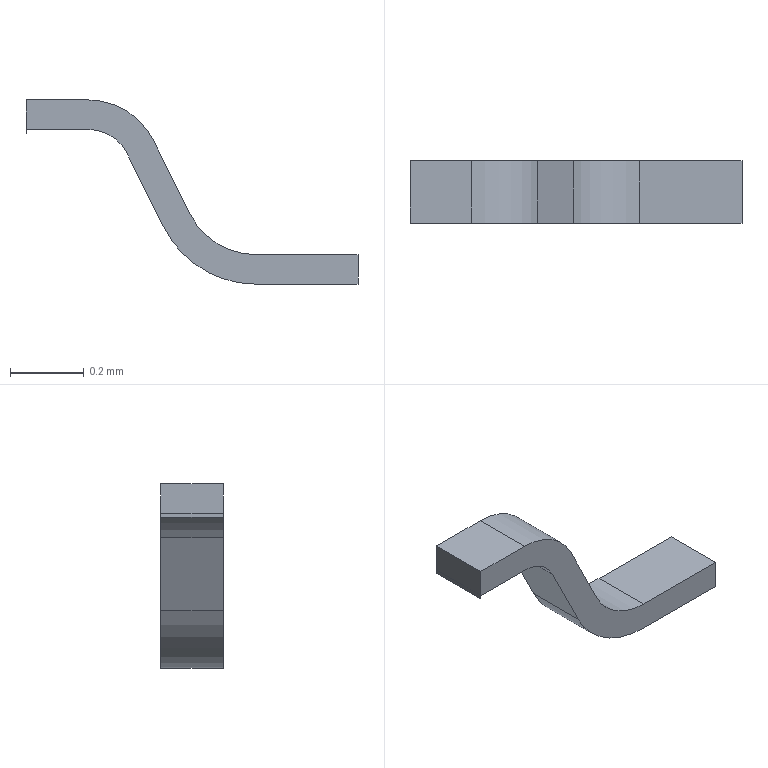Part | STEP file | RJ-USIO-V1_2-220411_6 | 1 solid | 15 faces | box 0.901 x 0.17 x 0.5 mm | volume 0.01509 mm3 | plane 11 | cylinder 4 | commonest cylinder face diameters 0.4 x2 0.24 x1 0.56 x1
STEP:
#1=CARTESIAN_POINT('',(0.,0.,0.));
#2=DIRECTION('',(0.,0.,1.));
#3=DIRECTION('',(1.,0.,0.));
#4=AXIS2_PLACEMENT_3D('',#1,#2,#3);
#5=CARTESIAN_POINT('',(55.657,51.036,0.5));
#6=VERTEX_POINT('',#5);
#7=CARTESIAN_POINT('',(55.657,50.866,0.5));
#8=VERTEX_POINT('',#7);
#9=CARTESIAN_POINT('',(55.657,51.036,0.5));
#10=DIRECTION('',(0.,-1.,0.));
#11=VECTOR('',#10,1.);
#12=LINE('',#9,#11);
#13=CARTESIAN_POINT('',(55.657,56.487,0.3));
#14=DIRECTION('',(0.,-1.,0.));
#15=DIRECTION('',(0.,0.,1.));
#16=AXIS2_PLACEMENT_3D('',#13,#14,#15);
#17=CYLINDRICAL_SURFACE('',#16,0.2);
#18=CARTESIAN_POINT('',(6.283,5.451));
#19=DIRECTION('',(0.,1.));
#20=VECTOR('',#19,1.);
#21=LINE('',#18,#20);
#22=(GEOMETRIC_REPRESENTATION_CONTEXT(2)PARAMETRIC_REPRESENTATION_CONTEXT()REPRESENTATION_CONTEXT('',''));
#23=DEFINITIONAL_REPRESENTATION('',(#21),#22);
#24=PCURVE('',#17,#23);
#25=CARTESIAN_POINT('',(56.39,50.866,0.5));
#26=DIRECTION('',(0.,0.,-1.));
#27=DIRECTION('',(1.,0.,0.));
#28=AXIS2_PLACEMENT_3D('',#25,#26,#27);
#29=PLANE('',#28);
#30=CARTESIAN_POINT('',(-0.7332,-0.17));
#31=DIRECTION('',(0.,1.));
#32=VECTOR('',#31,1.);
#33=LINE('',#30,#32);
#34=(GEOMETRIC_REPRESENTATION_CONTEXT(2)PARAMETRIC_REPRESENTATION_CONTEXT()REPRESENTATION_CONTEXT('',''));
#35=DEFINITIONAL_REPRESENTATION('',(#33),#34);
#36=PCURVE('',#29,#35);
#37=SURFACE_CURVE('',#12,(#24,#36),.PCURVE_S1.);
#38=EDGE_CURVE('',#6,#8,#37,.T.);
#39=ORIENTED_EDGE('',*,*,#38,.T.);
#40=CARTESIAN_POINT('',(55.836,50.866,0.3886));
#41=VERTEX_POINT('',#40);
#42=CARTESIAN_POINT('',(55.657,50.866,0.3));
#43=DIRECTION('',(0.,-1.,0.));
#44=DIRECTION('',(0.8964,0.,0.4432));
#45=AXIS2_PLACEMENT_3D('',#42,#43,#44);
#46=CIRCLE('',#45,0.2);
#47=CARTESIAN_POINT('',(5.172,5.621));
#48=DIRECTION('',(1.,0.));
#49=VECTOR('',#48,1.);
#50=LINE('',#47,#49);
#51=(GEOMETRIC_REPRESENTATION_CONTEXT(2)PARAMETRIC_REPRESENTATION_CONTEXT()REPRESENTATION_CONTEXT('',''));
#52=DEFINITIONAL_REPRESENTATION('',(#50),#51);
#53=PCURVE('',#17,#52);
#54=CARTESIAN_POINT('',(56.39,50.866,0.5));
#55=DIRECTION('',(0.,-1.,0.));
#56=DIRECTION('',(0.,0.,1.));
#57=AXIS2_PLACEMENT_3D('',#54,#55,#56);
#58=PLANE('',#57);
#59=CARTESIAN_POINT('',(-0.2,0.7332));
#60=DIRECTION('',(0.4432,-0.8964));
#61=AXIS2_PLACEMENT_2D('',#59,#60);
#62=CIRCLE('',#61,0.2);
#63=(GEOMETRIC_REPRESENTATION_CONTEXT(2)PARAMETRIC_REPRESENTATION_CONTEXT()REPRESENTATION_CONTEXT('',''));
#64=DEFINITIONAL_REPRESENTATION('',(#62),#63);
#65=PCURVE('',#58,#64);
#66=SURFACE_CURVE('',#46,(#53,#65),.PCURVE_S1.);
#67=EDGE_CURVE('',#41,#8,#66,.T.);
#68=ORIENTED_EDGE('',*,*,#67,.F.);
#69=CARTESIAN_POINT('',(55.836,51.036,0.3886));
#70=VERTEX_POINT('',#69);
#71=CARTESIAN_POINT('',(55.836,50.866,0.3886));
#72=DIRECTION('',(0.,1.,0.));
#73=VECTOR('',#72,1.);
#74=LINE('',#71,#73);
#75=CARTESIAN_POINT('',(5.172,5.621));
#76=DIRECTION('',(0.,-1.));
#77=VECTOR('',#76,1.);
#78=LINE('',#75,#77);
#79=(GEOMETRIC_REPRESENTATION_CONTEXT(2)PARAMETRIC_REPRESENTATION_CONTEXT()REPRESENTATION_CONTEXT('',''));
#80=DEFINITIONAL_REPRESENTATION('',(#78),#79);
#81=PCURVE('',#17,#80);
#82=CARTESIAN_POINT('',(55.934,56.487,0.1914));
#83=DIRECTION('',(-0.8964,0.,-0.4432));
#84=DIRECTION('',(0.4432,0.,-0.8964));
#85=AXIS2_PLACEMENT_3D('',#82,#83,#84);
#86=PLANE('',#85);
#87=CARTESIAN_POINT('',(-0.2201,5.621));
#88=DIRECTION('',(0.,-1.));
#89=VECTOR('',#88,1.);
#90=LINE('',#87,#89);
#91=(GEOMETRIC_REPRESENTATION_CONTEXT(2)PARAMETRIC_REPRESENTATION_CONTEXT()REPRESENTATION_CONTEXT('',''));
#92=DEFINITIONAL_REPRESENTATION('',(#90),#91);
#93=PCURVE('',#86,#92);
#94=SURFACE_CURVE('',#74,(#81,#93),.PCURVE_S1.);
#95=EDGE_CURVE('',#41,#70,#94,.T.);
#96=ORIENTED_EDGE('',*,*,#95,.T.);
#97=CARTESIAN_POINT('',(55.657,51.036,0.3));
#98=DIRECTION('',(0.,1.,0.));
#99=DIRECTION('',(0.,0.,1.));
#100=AXIS2_PLACEMENT_3D('',#97,#98,#99);
#101=CIRCLE('',#100,0.2);
#102=CARTESIAN_POINT('',(6.283,5.451));
#103=DIRECTION('',(-1.,0.));
#104=VECTOR('',#103,1.);
#105=LINE('',#102,#104);
#106=(GEOMETRIC_REPRESENTATION_CONTEXT(2)PARAMETRIC_REPRESENTATION_CONTEXT()REPRESENTATION_CONTEXT('',''));
#107=DEFINITIONAL_REPRESENTATION('',(#105),#106);
#108=PCURVE('',#17,#107);
#109=CARTESIAN_POINT('',(56.39,51.036,0.5));
#110=DIRECTION('',(0.,1.,0.));
#111=DIRECTION('',(0.,0.,-1.));
#112=AXIS2_PLACEMENT_3D('',#109,#110,#111);
#113=PLANE('',#112);
#114=CARTESIAN_POINT('',(0.2,0.7332));
#115=DIRECTION('',(-1.,0.));
#116=AXIS2_PLACEMENT_2D('',#114,#115);
#117=CIRCLE('',#116,0.2);
#118=(GEOMETRIC_REPRESENTATION_CONTEXT(2)PARAMETRIC_REPRESENTATION_CONTEXT()REPRESENTATION_CONTEXT('',''));
#119=DEFINITIONAL_REPRESENTATION('',(#117),#118);
#120=PCURVE('',#113,#119);
#121=SURFACE_CURVE('',#101,(#108,#120),.PCURVE_S1.);
#122=EDGE_CURVE('',#6,#70,#121,.T.);
#123=ORIENTED_EDGE('',*,*,#122,.F.);
#124=EDGE_LOOP('',(#39,#68,#96,#123));
#125=FACE_BOUND('',#124,.T.);
#126=ADVANCED_FACE('',(#125),#17,.T.);
#127=CARTESIAN_POINT('',(56.113,51.036,0.08));
#128=VERTEX_POINT('',#127);
#129=CARTESIAN_POINT('',(56.39,51.036,0.08));
#130=VERTEX_POINT('',#129);
#131=CARTESIAN_POINT('',(56.113,51.036,0.08));
#132=DIRECTION('',(1.,0.,0.));
#133=VECTOR('',#132,1.);
#134=LINE('',#131,#133);
#135=CARTESIAN_POINT('',(0.42,0.2771));
#136=DIRECTION('',(0.,-1.));
#137=VECTOR('',#136,1.);
#138=LINE('',#135,#137);
#139=(GEOMETRIC_REPRESENTATION_CONTEXT(2)PARAMETRIC_REPRESENTATION_CONTEXT()REPRESENTATION_CONTEXT('',''));
#140=DEFINITIONAL_REPRESENTATION('',(#138),#139);
#141=PCURVE('',#113,#140);
#142=CARTESIAN_POINT('',(56.39,56.487,0.08));
#143=DIRECTION('',(0.,0.,-1.));
#144=DIRECTION('',(1.,0.,0.));
#145=AXIS2_PLACEMENT_3D('',#142,#143,#144);
#146=PLANE('',#145);
#147=CARTESIAN_POINT('',(-0.2771,5.451));
#148=DIRECTION('',(1.,0.));
#149=VECTOR('',#148,1.);
#150=LINE('',#147,#149);
#151=(GEOMETRIC_REPRESENTATION_CONTEXT(2)PARAMETRIC_REPRESENTATION_CONTEXT()REPRESENTATION_CONTEXT('',''));
#152=DEFINITIONAL_REPRESENTATION('',(#150),#151);
#153=PCURVE('',#146,#152);
#154=SURFACE_CURVE('',#134,(#141,#153),.PCURVE_S1.);
#155=EDGE_CURVE('',#128,#130,#154,.T.);
#156=ORIENTED_EDGE('',*,*,#155,.F.);
#157=CARTESIAN_POINT('',(55.934,51.036,0.1914));
#158=VERTEX_POINT('',#157);
#159=CARTESIAN_POINT('',(56.113,51.036,0.28));
#160=DIRECTION('',(0.,-1.,0.));
#161=DIRECTION('',(-0.8964,0.,-0.4432));
#162=AXIS2_PLACEMENT_3D('',#159,#160,#161);
#163=CIRCLE('',#162,0.2);
#164=CARTESIAN_POINT('',(0.3086,0.4564));
#165=CARTESIAN_POINT('',(0.6192,0.3029));
#166=CARTESIAN_POINT('',(0.3309,0.1107));
#167=CARTESIAN_POINT('',(0.0427,-0.08145));
#168=CARTESIAN_POINT('',(0.02041,0.2642));
#169=CARTESIAN_POINT('',(-0.001873,0.6099));
#170=CARTESIAN_POINT('',(0.3086,0.4564));
#171=(BOUNDED_CURVE()B_SPLINE_CURVE(2,(#164,#165,#166,#167,#168,#169,#170),.UNSPECIFIED.,.T.,.F.)B_SPLINE_CURVE_WITH_KNOTS((1,2,2,2,2,1),(-2.094,0.,2.094,4.189,6.283,8.378),.UNSPECIFIED.)CURVE()GEOMETRIC_REPRESENTATION_ITEM()RATIONAL_B_SPLINE_CURVE((1.,0.5,1.,0.5,1.,0.5,1.))REPRESENTATION_ITEM(''));
#172=(GEOMETRIC_REPRESENTATION_CONTEXT(2)PARAMETRIC_REPRESENTATION_CONTEXT()REPRESENTATION_CONTEXT('',''));
#173=DEFINITIONAL_REPRESENTATION('',(#171),#172);
#174=PCURVE('',#113,#173);
#175=CARTESIAN_POINT('',(56.113,56.487,0.28));
#176=DIRECTION('',(0.,-1.,0.));
#177=DIRECTION('',(0.,0.,1.));
#178=AXIS2_PLACEMENT_3D('',#175,#176,#177);
#179=CYLINDRICAL_SURFACE('',#178,0.2);
#180=CARTESIAN_POINT('',(2.03,5.451));
#181=DIRECTION('',(1.,0.));
#182=VECTOR('',#181,1.);
#183=LINE('',#180,#182);
#184=(GEOMETRIC_REPRESENTATION_CONTEXT(2)PARAMETRIC_REPRESENTATION_CONTEXT()REPRESENTATION_CONTEXT('',''));
#185=DEFINITIONAL_REPRESENTATION('',(#183),#184);
#186=PCURVE('',#179,#185);
#187=SURFACE_CURVE('',#163,(#174,#186),.PCURVE_S1.);
#188=EDGE_CURVE('',#158,#128,#187,.T.);
#189=ORIENTED_EDGE('',*,*,#188,.F.);
#190=CARTESIAN_POINT('',(55.836,51.036,0.3886));
#191=DIRECTION('',(0.4432,0.,-0.8964));
#192=VECTOR('',#191,1.);
#193=LINE('',#190,#192);
#194=CARTESIAN_POINT('',(0.1114,0.554));
#195=DIRECTION('',(0.8964,-0.4432));
#196=VECTOR('',#195,1.);
#197=LINE('',#194,#196);
#198=(GEOMETRIC_REPRESENTATION_CONTEXT(2)PARAMETRIC_REPRESENTATION_CONTEXT()REPRESENTATION_CONTEXT('',''));
#199=DEFINITIONAL_REPRESENTATION('',(#197),#198);
#200=PCURVE('',#113,#199);
#201=CARTESIAN_POINT('',(-0.2201,5.451));
#202=DIRECTION('',(1.,0.));
#203=VECTOR('',#202,1.);
#204=LINE('',#201,#203);
#205=(GEOMETRIC_REPRESENTATION_CONTEXT(2)PARAMETRIC_REPRESENTATION_CONTEXT()REPRESENTATION_CONTEXT('',''));
#206=DEFINITIONAL_REPRESENTATION('',(#204),#205);
#207=PCURVE('',#86,#206);
#208=SURFACE_CURVE('',#193,(#200,#207),.PCURVE_S1.);
#209=EDGE_CURVE('',#70,#158,#208,.T.);
#210=ORIENTED_EDGE('',*,*,#209,.F.);
#211=ORIENTED_EDGE('',*,*,#122,.F.);
#212=CARTESIAN_POINT('',(55.489,51.036,0.5));
#213=VERTEX_POINT('',#212);
#214=CARTESIAN_POINT('',(55.657,51.036,0.5));
#215=DIRECTION('',(-1.,0.,0.));
#216=VECTOR('',#215,1.);
#217=LINE('',#214,#216);
#218=CARTESIAN_POINT('',(0.,0.7332));
#219=DIRECTION('',(0.,1.));
#220=VECTOR('',#219,1.);
#221=LINE('',#218,#220);
#222=(GEOMETRIC_REPRESENTATION_CONTEXT(2)PARAMETRIC_REPRESENTATION_CONTEXT()REPRESENTATION_CONTEXT('',''));
#223=DEFINITIONAL_REPRESENTATION('',(#221),#222);
#224=PCURVE('',#113,#223);
#225=CARTESIAN_POINT('',(-0.7332,-0.17));
#226=DIRECTION('',(-1.,0.));
#227=VECTOR('',#226,1.);
#228=LINE('',#225,#227);
#229=(GEOMETRIC_REPRESENTATION_CONTEXT(2)PARAMETRIC_REPRESENTATION_CONTEXT()REPRESENTATION_CONTEXT('',''));
#230=DEFINITIONAL_REPRESENTATION('',(#228),#229);
#231=PCURVE('',#29,#230);
#232=SURFACE_CURVE('',#217,(#224,#231),.PCURVE_S1.);
#233=EDGE_CURVE('',#6,#213,#232,.T.);
#234=ORIENTED_EDGE('',*,*,#233,.T.);
#235=CARTESIAN_POINT('',(55.489,51.036,0.4096));
#236=VERTEX_POINT('',#235);
#237=CARTESIAN_POINT('',(55.489,51.036,0.4096));
#238=DIRECTION('',(0.,0.,1.));
#239=VECTOR('',#238,1.);
#240=LINE('',#237,#239);
#241=CARTESIAN_POINT('',(0.09045,0.901));
#242=DIRECTION('',(-1.,0.));
#243=VECTOR('',#242,1.);
#244=LINE('',#241,#243);
#245=(GEOMETRIC_REPRESENTATION_CONTEXT(2)PARAMETRIC_REPRESENTATION_CONTEXT()REPRESENTATION_CONTEXT('',''));
#246=DEFINITIONAL_REPRESENTATION('',(#244),#245);
#247=PCURVE('',#113,#246);
#248=CARTESIAN_POINT('',(55.489,51.036,0.5));
#249=DIRECTION('',(-1.,0.,0.));
#250=DIRECTION('',(0.,0.,-1.));
#251=AXIS2_PLACEMENT_3D('',#248,#249,#250);
#252=PLANE('',#251);
#253=CARTESIAN_POINT('',(0.09045,0.));
#254=DIRECTION('',(-1.,0.));
#255=VECTOR('',#254,1.);
#256=LINE('',#253,#255);
#257=(GEOMETRIC_REPRESENTATION_CONTEXT(2)PARAMETRIC_REPRESENTATION_CONTEXT()REPRESENTATION_CONTEXT('',''));
#258=DEFINITIONAL_REPRESENTATION('',(#256),#257);
#259=PCURVE('',#252,#258);
#260=SURFACE_CURVE('',#240,(#247,#259),.PCURVE_S1.);
#261=EDGE_CURVE('',#236,#213,#260,.T.);
#262=ORIENTED_EDGE('',*,*,#261,.F.);
#263=CARTESIAN_POINT('',(55.49,51.036,0.42));
#264=VERTEX_POINT('',#263);
#265=CARTESIAN_POINT('',(55.49,51.036,0.42));
#266=DIRECTION('',(-0.1219,0.,-0.9925));
#267=VECTOR('',#266,1.);
#268=LINE('',#265,#267);
#269=CARTESIAN_POINT('',(0.08,0.8998));
#270=DIRECTION('',(0.9925,0.1219));
#271=VECTOR('',#270,1.);
#272=LINE('',#269,#271);
#273=(GEOMETRIC_REPRESENTATION_CONTEXT(2)PARAMETRIC_REPRESENTATION_CONTEXT()REPRESENTATION_CONTEXT('',''));
#274=DEFINITIONAL_REPRESENTATION('',(#272),#273);
#275=PCURVE('',#113,#274);
#276=CARTESIAN_POINT('',(55.49,56.487,0.42));
#277=DIRECTION('',(-0.9925,0.,0.1219));
#278=DIRECTION('',(-0.1219,0.,-0.9925));
#279=AXIS2_PLACEMENT_3D('',#276,#277,#278);
#280=PLANE('',#279);
#281=CARTESIAN_POINT('',(0.,5.451));
#282=DIRECTION('',(1.,0.));
#283=VECTOR('',#282,1.);
#284=LINE('',#281,#283);
#285=(GEOMETRIC_REPRESENTATION_CONTEXT(2)PARAMETRIC_REPRESENTATION_CONTEXT()REPRESENTATION_CONTEXT('',''));
#286=DEFINITIONAL_REPRESENTATION('',(#284),#285);
#287=PCURVE('',#280,#286);
#288=SURFACE_CURVE('',#268,(#275,#287),.PCURVE_S1.);
#289=EDGE_CURVE('',#264,#236,#288,.T.);
#290=ORIENTED_EDGE('',*,*,#289,.F.);
#291=CARTESIAN_POINT('',(55.657,51.036,0.42));
#292=VERTEX_POINT('',#291);
#293=CARTESIAN_POINT('',(55.657,51.036,0.42));
#294=DIRECTION('',(-1.,0.,0.));
#295=VECTOR('',#294,1.);
#296=LINE('',#293,#295);
#297=CARTESIAN_POINT('',(0.08,0.7332));
#298=DIRECTION('',(0.,1.));
#299=VECTOR('',#298,1.);
#300=LINE('',#297,#299);
#301=(GEOMETRIC_REPRESENTATION_CONTEXT(2)PARAMETRIC_REPRESENTATION_CONTEXT()REPRESENTATION_CONTEXT('',''));
#302=DEFINITIONAL_REPRESENTATION('',(#300),#301);
#303=PCURVE('',#113,#302);
#304=CARTESIAN_POINT('',(55.657,56.487,0.42));
#305=DIRECTION('',(0.,0.,1.));
#306=DIRECTION('',(-1.,0.,0.));
#307=AXIS2_PLACEMENT_3D('',#304,#305,#306);
#308=PLANE('',#307);
#309=CARTESIAN_POINT('',(0.,5.451));
#310=DIRECTION('',(1.,0.));
#311=VECTOR('',#310,1.);
#312=LINE('',#309,#311);
#313=(GEOMETRIC_REPRESENTATION_CONTEXT(2)PARAMETRIC_REPRESENTATION_CONTEXT()REPRESENTATION_CONTEXT('',''));
#314=DEFINITIONAL_REPRESENTATION('',(#312),#313);
#315=PCURVE('',#308,#314);
#316=SURFACE_CURVE('',#296,(#303,#315),.PCURVE_S1.);
#317=EDGE_CURVE('',#292,#264,#316,.T.);
#318=ORIENTED_EDGE('',*,*,#317,.F.);
#319=CARTESIAN_POINT('',(55.764,51.036,0.3532));
#320=VERTEX_POINT('',#319);
#321=CARTESIAN_POINT('',(55.657,51.036,0.3));
#322=DIRECTION('',(0.,-1.,0.));
#323=DIRECTION('',(0.8964,0.,0.4432));
#324=AXIS2_PLACEMENT_3D('',#321,#322,#323);
#325=CIRCLE('',#324,0.12);
#326=CARTESIAN_POINT('',(0.1468,0.6257));
#327=CARTESIAN_POINT('',(-0.0395,0.7178));
#328=CARTESIAN_POINT('',(0.1334,0.8331));
#329=CARTESIAN_POINT('',(0.3064,0.9484));
#330=CARTESIAN_POINT('',(0.3198,0.741));
#331=CARTESIAN_POINT('',(0.3331,0.5335));
#332=CARTESIAN_POINT('',(0.1468,0.6257));
#333=(BOUNDED_CURVE()B_SPLINE_CURVE(2,(#326,#327,#328,#329,#330,#331,#332),.UNSPECIFIED.,.T.,.F.)B_SPLINE_CURVE_WITH_KNOTS((1,2,2,2,2,1),(-2.094,0.,2.094,4.189,6.283,8.378),.UNSPECIFIED.)CURVE()GEOMETRIC_REPRESENTATION_ITEM()RATIONAL_B_SPLINE_CURVE((1.,0.5,1.,0.5,1.,0.5,1.))REPRESENTATION_ITEM(''));
#334=(GEOMETRIC_REPRESENTATION_CONTEXT(2)PARAMETRIC_REPRESENTATION_CONTEXT()REPRESENTATION_CONTEXT('',''));
#335=DEFINITIONAL_REPRESENTATION('',(#333),#334);
#336=PCURVE('',#113,#335);
#337=CARTESIAN_POINT('',(55.657,56.487,0.3));
#338=DIRECTION('',(0.,-1.,0.));
#339=DIRECTION('',(0.,0.,1.));
#340=AXIS2_PLACEMENT_3D('',#337,#338,#339);
#341=CYLINDRICAL_SURFACE('',#340,0.12);
#342=CARTESIAN_POINT('',(5.172,5.451));
#343=DIRECTION('',(1.,0.));
#344=VECTOR('',#343,1.);
#345=LINE('',#342,#344);
#346=(GEOMETRIC_REPRESENTATION_CONTEXT(2)PARAMETRIC_REPRESENTATION_CONTEXT()REPRESENTATION_CONTEXT('',''));
#347=DEFINITIONAL_REPRESENTATION('',(#345),#346);
#348=PCURVE('',#341,#347);
#349=SURFACE_CURVE('',#325,(#336,#348),.PCURVE_S1.);
#350=EDGE_CURVE('',#320,#292,#349,.T.);
#351=ORIENTED_EDGE('',*,*,#350,.F.);
#352=CARTESIAN_POINT('',(55.862,51.036,0.1559));
#353=VERTEX_POINT('',#352);
#354=CARTESIAN_POINT('',(55.862,51.036,0.1559));
#355=DIRECTION('',(-0.4432,0.,0.8964));
#356=VECTOR('',#355,1.);
#357=LINE('',#354,#356);
#358=CARTESIAN_POINT('',(0.3441,0.5281));
#359=DIRECTION('',(-0.8964,0.4432));
#360=VECTOR('',#359,1.);
#361=LINE('',#358,#360);
#362=(GEOMETRIC_REPRESENTATION_CONTEXT(2)PARAMETRIC_REPRESENTATION_CONTEXT()REPRESENTATION_CONTEXT('',''));
#363=DEFINITIONAL_REPRESENTATION('',(#361),#362);
#364=PCURVE('',#113,#363);
#365=CARTESIAN_POINT('',(55.862,56.487,0.1559));
#366=DIRECTION('',(0.8964,0.,0.4432));
#367=DIRECTION('',(-0.4432,0.,0.8964));
#368=AXIS2_PLACEMENT_3D('',#365,#366,#367);
#369=PLANE('',#368);
#370=CARTESIAN_POINT('',(0.,5.451));
#371=DIRECTION('',(1.,0.));
#372=VECTOR('',#371,1.);
#373=LINE('',#370,#372);
#374=(GEOMETRIC_REPRESENTATION_CONTEXT(2)PARAMETRIC_REPRESENTATION_CONTEXT()REPRESENTATION_CONTEXT('',''));
#375=DEFINITIONAL_REPRESENTATION('',(#373),#374);
#376=PCURVE('',#369,#375);
#377=SURFACE_CURVE('',#357,(#364,#376),.PCURVE_S1.);
#378=EDGE_CURVE('',#353,#320,#377,.T.);
#379=ORIENTED_EDGE('',*,*,#378,.F.);
#380=CARTESIAN_POINT('',(56.113,51.036,0.));
#381=VERTEX_POINT('',#380);
#382=CARTESIAN_POINT('',(56.113,51.036,0.28));
#383=DIRECTION('',(0.,1.,0.));
#384=DIRECTION('',(0.,0.,-1.));
#385=AXIS2_PLACEMENT_3D('',#382,#383,#384);
#386=CIRCLE('',#385,0.28);
#387=CARTESIAN_POINT('',(0.22,0.2771));
#388=DIRECTION('',(1.,0.));
#389=AXIS2_PLACEMENT_2D('',#387,#388);
#390=CIRCLE('',#389,0.28);
#391=(GEOMETRIC_REPRESENTATION_CONTEXT(2)PARAMETRIC_REPRESENTATION_CONTEXT()REPRESENTATION_CONTEXT('',''));
#392=DEFINITIONAL_REPRESENTATION('',(#390),#391);
#393=PCURVE('',#113,#392);
#394=CARTESIAN_POINT('',(56.113,56.487,0.28));
#395=DIRECTION('',(0.,-1.,0.));
#396=DIRECTION('',(0.,0.,1.));
#397=AXIS2_PLACEMENT_3D('',#394,#395,#396);
#398=CYLINDRICAL_SURFACE('',#397,0.28);
#399=CARTESIAN_POINT('',(3.142,5.451));
#400=DIRECTION('',(-1.,0.));
#401=VECTOR('',#400,1.);
#402=LINE('',#399,#401);
#403=(GEOMETRIC_REPRESENTATION_CONTEXT(2)PARAMETRIC_REPRESENTATION_CONTEXT()REPRESENTATION_CONTEXT('',''));
#404=DEFINITIONAL_REPRESENTATION('',(#402),#403);
#405=PCURVE('',#398,#404);
#406=SURFACE_CURVE('',#386,(#393,#405),.PCURVE_S1.);
#407=EDGE_CURVE('',#381,#353,#406,.T.);
#408=ORIENTED_EDGE('',*,*,#407,.F.);
#409=CARTESIAN_POINT('',(56.39,51.036,0.));
#410=VERTEX_POINT('',#409);
#411=CARTESIAN_POINT('',(56.39,51.036,0.));
#412=DIRECTION('',(-1.,0.,0.));
#413=VECTOR('',#412,1.);
#414=LINE('',#411,#413);
#415=CARTESIAN_POINT('',(0.5,0.));
#416=DIRECTION('',(0.,1.));
#417=VECTOR('',#416,1.);
#418=LINE('',#415,#417);
#419=(GEOMETRIC_REPRESENTATION_CONTEXT(2)PARAMETRIC_REPRESENTATION_CONTEXT()REPRESENTATION_CONTEXT('',''));
#420=DEFINITIONAL_REPRESENTATION('',(#418),#419);
#421=PCURVE('',#113,#420);
#422=CARTESIAN_POINT('',(56.39,50.866,0.));
#423=DIRECTION('',(0.,0.,-1.));
#424=DIRECTION('',(1.,0.,0.));
#425=AXIS2_PLACEMENT_3D('',#422,#423,#424);
#426=PLANE('',#425);
#427=CARTESIAN_POINT('',(0.,-0.17));
#428=DIRECTION('',(-1.,0.));
#429=VECTOR('',#428,1.);
#430=LINE('',#427,#429);
#431=(GEOMETRIC_REPRESENTATION_CONTEXT(2)PARAMETRIC_REPRESENTATION_CONTEXT()REPRESENTATION_CONTEXT('',''));
#432=DEFINITIONAL_REPRESENTATION('',(#430),#431);
#433=PCURVE('',#426,#432);
#434=SURFACE_CURVE('',#414,(#421,#433),.PCURVE_S1.);
#435=EDGE_CURVE('',#410,#381,#434,.T.);
#436=ORIENTED_EDGE('',*,*,#435,.F.);
#437=CARTESIAN_POINT('',(56.39,51.036,0.));
#438=DIRECTION('',(0.,0.,1.));
#439=VECTOR('',#438,1.);
#440=LINE('',#437,#439);
#441=CARTESIAN_POINT('',(0.5,0.));
#442=DIRECTION('',(-1.,0.));
#443=VECTOR('',#442,1.);
#444=LINE('',#441,#443);
#445=(GEOMETRIC_REPRESENTATION_CONTEXT(2)PARAMETRIC_REPRESENTATION_CONTEXT()REPRESENTATION_CONTEXT('',''));
#446=DEFINITIONAL_REPRESENTATION('',(#444),#445);
#447=PCURVE('',#113,#446);
#448=CARTESIAN_POINT('',(56.39,51.036,0.5));
#449=DIRECTION('',(1.,0.,0.));
#450=DIRECTION('',(0.,0.,1.));
#451=AXIS2_PLACEMENT_3D('',#448,#449,#450);
#452=PLANE('',#451);
#453=CARTESIAN_POINT('',(-0.5,0.));
#454=DIRECTION('',(1.,0.));
#455=VECTOR('',#454,1.);
#456=LINE('',#453,#455);
#457=(GEOMETRIC_REPRESENTATION_CONTEXT(2)PARAMETRIC_REPRESENTATION_CONTEXT()REPRESENTATION_CONTEXT('',''));
#458=DEFINITIONAL_REPRESENTATION('',(#456),#457);
#459=PCURVE('',#452,#458);
#460=SURFACE_CURVE('',#440,(#447,#459),.PCURVE_S1.);
#461=EDGE_CURVE('',#410,#130,#460,.T.);
#462=ORIENTED_EDGE('',*,*,#461,.T.);
#463=EDGE_LOOP('',(#156,#189,#210,#211,#234,#262,#290,#318,#351,#379,#408,#436,#462));
#464=FACE_BOUND('',#463,.F.);
#465=ADVANCED_FACE('',(#464),#113,.T.);
#466=ORIENTED_EDGE('',*,*,#155,.T.);
#467=CARTESIAN_POINT('',(56.39,50.866,0.08));
#468=VERTEX_POINT('',#467);
#469=CARTESIAN_POINT('',(56.39,50.866,0.08));
#470=DIRECTION('',(0.,1.,0.));
#471=VECTOR('',#470,1.);
#472=LINE('',#469,#471);
#473=CARTESIAN_POINT('',(0.,5.621));
#474=DIRECTION('',(0.,-1.));
#475=VECTOR('',#474,1.);
#476=LINE('',#473,#475);
#477=(GEOMETRIC_REPRESENTATION_CONTEXT(2)PARAMETRIC_REPRESENTATION_CONTEXT()REPRESENTATION_CONTEXT('',''));
#478=DEFINITIONAL_REPRESENTATION('',(#476),#477);
#479=PCURVE('',#146,#478);
#480=CARTESIAN_POINT('',(-0.42,0.17));
#481=DIRECTION('',(0.,-1.));
#482=VECTOR('',#481,1.);
#483=LINE('',#480,#482);
#484=(GEOMETRIC_REPRESENTATION_CONTEXT(2)PARAMETRIC_REPRESENTATION_CONTEXT()REPRESENTATION_CONTEXT('',''));
#485=DEFINITIONAL_REPRESENTATION('',(#483),#484);
#486=PCURVE('',#452,#485);
#487=SURFACE_CURVE('',#472,(#479,#486),.PCURVE_S1.);
#488=EDGE_CURVE('',#468,#130,#487,.T.);
#489=ORIENTED_EDGE('',*,*,#488,.F.);
#490=CARTESIAN_POINT('',(56.113,50.866,0.08));
#491=VERTEX_POINT('',#490);
#492=CARTESIAN_POINT('',(56.39,50.866,0.08));
#493=DIRECTION('',(-1.,0.,0.));
#494=VECTOR('',#493,1.);
#495=LINE('',#492,#494);
#496=CARTESIAN_POINT('',(0.,5.621));
#497=DIRECTION('',(-1.,0.));
#498=VECTOR('',#497,1.);
#499=LINE('',#496,#498);
#500=(GEOMETRIC_REPRESENTATION_CONTEXT(2)PARAMETRIC_REPRESENTATION_CONTEXT()REPRESENTATION_CONTEXT('',''));
#501=DEFINITIONAL_REPRESENTATION('',(#499),#500);
#502=PCURVE('',#146,#501);
#503=CARTESIAN_POINT('',(-0.42,0.));
#504=DIRECTION('',(0.,1.));
#505=VECTOR('',#504,1.);
#506=LINE('',#503,#505);
#507=(GEOMETRIC_REPRESENTATION_CONTEXT(2)PARAMETRIC_REPRESENTATION_CONTEXT()REPRESENTATION_CONTEXT('',''));
#508=DEFINITIONAL_REPRESENTATION('',(#506),#507);
#509=PCURVE('',#58,#508);
#510=SURFACE_CURVE('',#495,(#502,#509),.PCURVE_S1.);
#511=EDGE_CURVE('',#468,#491,#510,.T.);
#512=ORIENTED_EDGE('',*,*,#511,.T.);
#513=CARTESIAN_POINT('',(56.113,50.866,0.08));
#514=DIRECTION('',(0.,1.,0.));
#515=VECTOR('',#514,1.);
#516=LINE('',#513,#515);
#517=CARTESIAN_POINT('',(-0.2771,5.621));
#518=DIRECTION('',(0.,-1.));
#519=VECTOR('',#518,1.);
#520=LINE('',#517,#519);
#521=(GEOMETRIC_REPRESENTATION_CONTEXT(2)PARAMETRIC_REPRESENTATION_CONTEXT()REPRESENTATION_CONTEXT('',''));
#522=DEFINITIONAL_REPRESENTATION('',(#520),#521);
#523=PCURVE('',#146,#522);
#524=CARTESIAN_POINT('',(3.142,5.621));
#525=DIRECTION('',(0.,-1.));
#526=VECTOR('',#525,1.);
#527=LINE('',#524,#526);
#528=(GEOMETRIC_REPRESENTATION_CONTEXT(2)PARAMETRIC_REPRESENTATION_CONTEXT()REPRESENTATION_CONTEXT('',''));
#529=DEFINITIONAL_REPRESENTATION('',(#527),#528);
#530=PCURVE('',#179,#529);
#531=SURFACE_CURVE('',#516,(#523,#530),.PCURVE_S1.);
#532=EDGE_CURVE('',#491,#128,#531,.T.);
#533=ORIENTED_EDGE('',*,*,#532,.T.);
#534=EDGE_LOOP('',(#466,#489,#512,#533));
#535=FACE_BOUND('',#534,.F.);
#536=ADVANCED_FACE('',(#535),#146,.F.);
#537=ORIENTED_EDGE('',*,*,#488,.T.);
#538=ORIENTED_EDGE('',*,*,#461,.F.);
#539=CARTESIAN_POINT('',(56.39,50.866,0.));
#540=VERTEX_POINT('',#539);
#541=CARTESIAN_POINT('',(56.39,50.866,0.));
#542=DIRECTION('',(0.,1.,0.));
#543=VECTOR('',#542,1.);
#544=LINE('',#541,#543);
#545=CARTESIAN_POINT('',(-0.5,0.17));
#546=DIRECTION('',(0.,-1.));
#547=VECTOR('',#546,1.);
#548=LINE('',#545,#547);
#549=(GEOMETRIC_REPRESENTATION_CONTEXT(2)PARAMETRIC_REPRESENTATION_CONTEXT()REPRESENTATION_CONTEXT('',''));
#550=DEFINITIONAL_REPRESENTATION('',(#548),#549);
#551=PCURVE('',#452,#550);
#552=CARTESIAN_POINT('',(0.,0.));
#553=DIRECTION('',(0.,-1.));
#554=VECTOR('',#553,1.);
#555=LINE('',#552,#554);
#556=(GEOMETRIC_REPRESENTATION_CONTEXT(2)PARAMETRIC_REPRESENTATION_CONTEXT()REPRESENTATION_CONTEXT('',''));
#557=DEFINITIONAL_REPRESENTATION('',(#555),#556);
#558=PCURVE('',#426,#557);
#559=SURFACE_CURVE('',#544,(#551,#558),.PCURVE_S1.);
#560=EDGE_CURVE('',#540,#410,#559,.T.);
#561=ORIENTED_EDGE('',*,*,#560,.F.);
#562=CARTESIAN_POINT('',(56.39,50.866,0.));
#563=DIRECTION('',(0.,0.,1.));
#564=VECTOR('',#563,1.);
#565=LINE('',#562,#564);
#566=CARTESIAN_POINT('',(-0.5,0.17));
#567=DIRECTION('',(1.,0.));
#568=VECTOR('',#567,1.);
#569=LINE('',#566,#568);
#570=(GEOMETRIC_REPRESENTATION_CONTEXT(2)PARAMETRIC_REPRESENTATION_CONTEXT()REPRESENTATION_CONTEXT('',''));
#571=DEFINITIONAL_REPRESENTATION('',(#569),#570);
#572=PCURVE('',#452,#571);
#573=CARTESIAN_POINT('',(-0.5,0.));
#574=DIRECTION('',(1.,0.));
#575=VECTOR('',#574,1.);
#576=LINE('',#573,#575);
#577=(GEOMETRIC_REPRESENTATION_CONTEXT(2)PARAMETRIC_REPRESENTATION_CONTEXT()REPRESENTATION_CONTEXT('',''));
#578=DEFINITIONAL_REPRESENTATION('',(#576),#577);
#579=PCURVE('',#58,#578);
#580=SURFACE_CURVE('',#565,(#572,#579),.PCURVE_S1.);
#581=EDGE_CURVE('',#540,#468,#580,.T.);
#582=ORIENTED_EDGE('',*,*,#581,.T.);
#583=EDGE_LOOP('',(#537,#538,#561,#582));
#584=FACE_BOUND('',#583,.F.);
#585=ADVANCED_FACE('',(#584),#452,.T.);
#586=CARTESIAN_POINT('',(56.113,50.866,0.));
#587=VERTEX_POINT('',#586);
#588=CARTESIAN_POINT('',(56.113,50.866,0.));
#589=DIRECTION('',(1.,0.,0.));
#590=VECTOR('',#589,1.);
#591=LINE('',#588,#590);
#592=CARTESIAN_POINT('',(-0.2771,0.));
#593=DIRECTION('',(1.,0.));
#594=VECTOR('',#593,1.);
#595=LINE('',#592,#594);
#596=(GEOMETRIC_REPRESENTATION_CONTEXT(2)PARAMETRIC_REPRESENTATION_CONTEXT()REPRESENTATION_CONTEXT('',''));
#597=DEFINITIONAL_REPRESENTATION('',(#595),#596);
#598=PCURVE('',#426,#597);
#599=CARTESIAN_POINT('',(-0.5,0.2771));
#600=DIRECTION('',(0.,-1.));
#601=VECTOR('',#600,1.);
#602=LINE('',#599,#601);
#603=(GEOMETRIC_REPRESENTATION_CONTEXT(2)PARAMETRIC_REPRESENTATION_CONTEXT()REPRESENTATION_CONTEXT('',''));
#604=DEFINITIONAL_REPRESENTATION('',(#602),#603);
#605=PCURVE('',#58,#604);
#606=SURFACE_CURVE('',#591,(#598,#605),.PCURVE_S1.);
#607=EDGE_CURVE('',#587,#540,#606,.T.);
#608=ORIENTED_EDGE('',*,*,#607,.T.);
#609=ORIENTED_EDGE('',*,*,#560,.T.);
#610=ORIENTED_EDGE('',*,*,#435,.T.);
#611=CARTESIAN_POINT('',(56.113,51.036,0.));
#612=DIRECTION('',(0.,-1.,0.));
#613=VECTOR('',#612,1.);
#614=LINE('',#611,#613);
#615=CARTESIAN_POINT('',(-0.2771,-0.17));
#616=DIRECTION('',(0.,1.));
#617=VECTOR('',#616,1.);
#618=LINE('',#615,#617);
#619=(GEOMETRIC_REPRESENTATION_CONTEXT(2)PARAMETRIC_REPRESENTATION_CONTEXT()REPRESENTATION_CONTEXT('',''));
#620=DEFINITIONAL_REPRESENTATION('',(#618),#619);
#621=PCURVE('',#426,#620);
#622=CARTESIAN_POINT('',(3.142,5.451));
#623=DIRECTION('',(0.,1.));
#624=VECTOR('',#623,1.);
#625=LINE('',#622,#624);
#626=(GEOMETRIC_REPRESENTATION_CONTEXT(2)PARAMETRIC_REPRESENTATION_CONTEXT()REPRESENTATION_CONTEXT('',''));
#627=DEFINITIONAL_REPRESENTATION('',(#625),#626);
#628=PCURVE('',#398,#627);
#629=SURFACE_CURVE('',#614,(#621,#628),.PCURVE_S1.);
#630=EDGE_CURVE('',#381,#587,#629,.T.);
#631=ORIENTED_EDGE('',*,*,#630,.T.);
#632=EDGE_LOOP('',(#608,#609,#610,#631));
#633=FACE_BOUND('',#632,.F.);
#634=ADVANCED_FACE('',(#633),#426,.T.);
#635=ORIENTED_EDGE('',*,*,#511,.F.);
#636=ORIENTED_EDGE('',*,*,#581,.F.);
#637=ORIENTED_EDGE('',*,*,#607,.F.);
#638=CARTESIAN_POINT('',(55.862,50.866,0.1559));
#639=VERTEX_POINT('',#638);
#640=CARTESIAN_POINT('',(56.113,50.866,0.28));
#641=DIRECTION('',(0.,-1.,0.));
#642=DIRECTION('',(-0.8964,0.,-0.4432));
#643=AXIS2_PLACEMENT_3D('',#640,#641,#642);
#644=CIRCLE('',#643,0.28);
#645=CARTESIAN_POINT('',(-0.22,0.2771));
#646=DIRECTION('',(-0.4432,0.8964));
#647=AXIS2_PLACEMENT_2D('',#645,#646);
#648=CIRCLE('',#647,0.28);
#649=(GEOMETRIC_REPRESENTATION_CONTEXT(2)PARAMETRIC_REPRESENTATION_CONTEXT()REPRESENTATION_CONTEXT('',''));
#650=DEFINITIONAL_REPRESENTATION('',(#648),#649);
#651=PCURVE('',#58,#650);
#652=CARTESIAN_POINT('',(2.03,5.621));
#653=DIRECTION('',(1.,0.));
#654=VECTOR('',#653,1.);
#655=LINE('',#652,#654);
#656=(GEOMETRIC_REPRESENTATION_CONTEXT(2)PARAMETRIC_REPRESENTATION_CONTEXT()REPRESENTATION_CONTEXT('',''));
#657=DEFINITIONAL_REPRESENTATION('',(#655),#656);
#658=PCURVE('',#398,#657);
#659=SURFACE_CURVE('',#644,(#651,#658),.PCURVE_S1.);
#660=EDGE_CURVE('',#639,#587,#659,.T.);
#661=ORIENTED_EDGE('',*,*,#660,.F.);
#662=CARTESIAN_POINT('',(55.764,50.866,0.3532));
#663=VERTEX_POINT('',#662);
#664=CARTESIAN_POINT('',(55.764,50.866,0.3532));
#665=DIRECTION('',(0.4432,0.,-0.8964));
#666=VECTOR('',#665,1.);
#667=LINE('',#664,#666);
#668=CARTESIAN_POINT('',(-0.1468,0.6257));
#669=DIRECTION('',(-0.8964,-0.4432));
#670=VECTOR('',#669,1.);
#671=LINE('',#668,#670);
#672=(GEOMETRIC_REPRESENTATION_CONTEXT(2)PARAMETRIC_REPRESENTATION_CONTEXT()REPRESENTATION_CONTEXT('',''));
#673=DEFINITIONAL_REPRESENTATION('',(#671),#672);
#674=PCURVE('',#58,#673);
#675=CARTESIAN_POINT('',(0.2201,5.621));
#676=DIRECTION('',(-1.,0.));
#677=VECTOR('',#676,1.);
#678=LINE('',#675,#677);
#679=(GEOMETRIC_REPRESENTATION_CONTEXT(2)PARAMETRIC_REPRESENTATION_CONTEXT()REPRESENTATION_CONTEXT('',''));
#680=DEFINITIONAL_REPRESENTATION('',(#678),#679);
#681=PCURVE('',#369,#680);
#682=SURFACE_CURVE('',#667,(#674,#681),.PCURVE_S1.);
#683=EDGE_CURVE('',#663,#639,#682,.T.);
#684=ORIENTED_EDGE('',*,*,#683,.F.);
#685=CARTESIAN_POINT('',(55.657,50.866,0.42));
#686=VERTEX_POINT('',#685);
#687=CARTESIAN_POINT('',(55.657,50.866,0.3));
#688=DIRECTION('',(0.,1.,0.));
#689=DIRECTION('',(0.,0.,1.));
#690=AXIS2_PLACEMENT_3D('',#687,#688,#689);
#691=CIRCLE('',#690,0.12);
#692=CARTESIAN_POINT('',(-0.08,0.7332));
#693=CARTESIAN_POINT('',(-0.08,0.5254));
#694=CARTESIAN_POINT('',(-0.26,0.6293));
#695=CARTESIAN_POINT('',(-0.44,0.7332));
#696=CARTESIAN_POINT('',(-0.26,0.8372));
#697=CARTESIAN_POINT('',(-0.08,0.9411));
#698=CARTESIAN_POINT('',(-0.08,0.7332));
#699=(BOUNDED_CURVE()B_SPLINE_CURVE(2,(#692,#693,#694,#695,#696,#697,#698),.UNSPECIFIED.,.T.,.F.)B_SPLINE_CURVE_WITH_KNOTS((1,2,2,2,2,1),(-2.094,0.,2.094,4.189,6.283,8.378),.UNSPECIFIED.)CURVE()GEOMETRIC_REPRESENTATION_ITEM()RATIONAL_B_SPLINE_CURVE((1.,0.5,1.,0.5,1.,0.5,1.))REPRESENTATION_ITEM(''));
#700=(GEOMETRIC_REPRESENTATION_CONTEXT(2)PARAMETRIC_REPRESENTATION_CONTEXT()REPRESENTATION_CONTEXT('',''));
#701=DEFINITIONAL_REPRESENTATION('',(#699),#700);
#702=PCURVE('',#58,#701);
#703=CARTESIAN_POINT('',(6.283,5.621));
#704=DIRECTION('',(-1.,0.));
#705=VECTOR('',#704,1.);
#706=LINE('',#703,#705);
#707=(GEOMETRIC_REPRESENTATION_CONTEXT(2)PARAMETRIC_REPRESENTATION_CONTEXT()REPRESENTATION_CONTEXT('',''));
#708=DEFINITIONAL_REPRESENTATION('',(#706),#707);
#709=PCURVE('',#341,#708);
#710=SURFACE_CURVE('',#691,(#702,#709),.PCURVE_S1.);
#711=EDGE_CURVE('',#686,#663,#710,.T.);
#712=ORIENTED_EDGE('',*,*,#711,.F.);
#713=CARTESIAN_POINT('',(55.49,50.866,0.42));
#714=VERTEX_POINT('',#713);
#715=CARTESIAN_POINT('',(55.49,50.866,0.42));
#716=DIRECTION('',(1.,0.,0.));
#717=VECTOR('',#716,1.);
#718=LINE('',#715,#717);
#719=CARTESIAN_POINT('',(-0.08,0.8998));
#720=DIRECTION('',(0.,-1.));
#721=VECTOR('',#720,1.);
#722=LINE('',#719,#721);
#723=(GEOMETRIC_REPRESENTATION_CONTEXT(2)PARAMETRIC_REPRESENTATION_CONTEXT()REPRESENTATION_CONTEXT('',''));
#724=DEFINITIONAL_REPRESENTATION('',(#722),#723);
#725=PCURVE('',#58,#724);
#726=CARTESIAN_POINT('',(0.1665,5.621));
#727=DIRECTION('',(-1.,0.));
#728=VECTOR('',#727,1.);
#729=LINE('',#726,#728);
#730=(GEOMETRIC_REPRESENTATION_CONTEXT(2)PARAMETRIC_REPRESENTATION_CONTEXT()REPRESENTATION_CONTEXT('',''));
#731=DEFINITIONAL_REPRESENTATION('',(#729),#730);
#732=PCURVE('',#308,#731);
#733=SURFACE_CURVE('',#718,(#725,#732),.PCURVE_S1.);
#734=EDGE_CURVE('',#714,#686,#733,.T.);
#735=ORIENTED_EDGE('',*,*,#734,.F.);
#736=CARTESIAN_POINT('',(55.489,50.866,0.4096));
#737=VERTEX_POINT('',#736);
#738=CARTESIAN_POINT('',(55.489,50.866,0.4096));
#739=DIRECTION('',(0.1219,0.,0.9925));
#740=VECTOR('',#739,1.);
#741=LINE('',#738,#740);
#742=CARTESIAN_POINT('',(-0.09045,0.901));
#743=DIRECTION('',(0.9925,-0.1219));
#744=VECTOR('',#743,1.);
#745=LINE('',#742,#744);
#746=(GEOMETRIC_REPRESENTATION_CONTEXT(2)PARAMETRIC_REPRESENTATION_CONTEXT()REPRESENTATION_CONTEXT('',''));
#747=DEFINITIONAL_REPRESENTATION('',(#745),#746);
#748=PCURVE('',#58,#747);
#749=CARTESIAN_POINT('',(0.01053,5.621));
#750=DIRECTION('',(-1.,0.));
#751=VECTOR('',#750,1.);
#752=LINE('',#749,#751);
#753=(GEOMETRIC_REPRESENTATION_CONTEXT(2)PARAMETRIC_REPRESENTATION_CONTEXT()REPRESENTATION_CONTEXT('',''));
#754=DEFINITIONAL_REPRESENTATION('',(#752),#753);
#755=PCURVE('',#280,#754);
#756=SURFACE_CURVE('',#741,(#748,#755),.PCURVE_S1.);
#757=EDGE_CURVE('',#737,#714,#756,.T.);
#758=ORIENTED_EDGE('',*,*,#757,.F.);
#759=CARTESIAN_POINT('',(55.489,50.866,0.5));
#760=VERTEX_POINT('',#759);
#761=CARTESIAN_POINT('',(55.489,50.866,0.4096));
#762=DIRECTION('',(0.,0.,1.));
#763=VECTOR('',#762,1.);
#764=LINE('',#761,#763);
#765=CARTESIAN_POINT('',(-0.09045,0.901));
#766=DIRECTION('',(1.,0.));
#767=VECTOR('',#766,1.);
#768=LINE('',#765,#767);
#769=(GEOMETRIC_REPRESENTATION_CONTEXT(2)PARAMETRIC_REPRESENTATION_CONTEXT()REPRESENTATION_CONTEXT('',''));
#770=DEFINITIONAL_REPRESENTATION('',(#768),#769);
#771=PCURVE('',#58,#770);
#772=CARTESIAN_POINT('',(0.09045,0.17));
#773=DIRECTION('',(-1.,0.));
#774=VECTOR('',#773,1.);
#775=LINE('',#772,#774);
#776=(GEOMETRIC_REPRESENTATION_CONTEXT(2)PARAMETRIC_REPRESENTATION_CONTEXT()REPRESENTATION_CONTEXT('',''));
#777=DEFINITIONAL_REPRESENTATION('',(#775),#776);
#778=PCURVE('',#252,#777);
#779=SURFACE_CURVE('',#764,(#771,#778),.PCURVE_S1.);
#780=EDGE_CURVE('',#737,#760,#779,.T.);
#781=ORIENTED_EDGE('',*,*,#780,.T.);
#782=CARTESIAN_POINT('',(55.489,50.866,0.5));
#783=DIRECTION('',(1.,0.,0.));
#784=VECTOR('',#783,1.);
#785=LINE('',#782,#784);
#786=CARTESIAN_POINT('',(0.,0.901));
#787=DIRECTION('',(0.,-1.));
#788=VECTOR('',#787,1.);
#789=LINE('',#786,#788);
#790=(GEOMETRIC_REPRESENTATION_CONTEXT(2)PARAMETRIC_REPRESENTATION_CONTEXT()REPRESENTATION_CONTEXT('',''));
#791=DEFINITIONAL_REPRESENTATION('',(#789),#790);
#792=PCURVE('',#58,#791);
#793=CARTESIAN_POINT('',(-0.901,0.));
#794=DIRECTION('',(1.,0.));
#795=VECTOR('',#794,1.);
#796=LINE('',#793,#795);
#797=(GEOMETRIC_REPRESENTATION_CONTEXT(2)PARAMETRIC_REPRESENTATION_CONTEXT()REPRESENTATION_CONTEXT('',''));
#798=DEFINITIONAL_REPRESENTATION('',(#796),#797);
#799=PCURVE('',#29,#798);
#800=SURFACE_CURVE('',#785,(#792,#799),.PCURVE_S1.);
#801=EDGE_CURVE('',#760,#8,#800,.T.);
#802=ORIENTED_EDGE('',*,*,#801,.T.);
#803=ORIENTED_EDGE('',*,*,#67,.F.);
#804=CARTESIAN_POINT('',(55.934,50.866,0.1914));
#805=VERTEX_POINT('',#804);
#806=CARTESIAN_POINT('',(55.934,50.866,0.1914));
#807=DIRECTION('',(-0.4432,0.,0.8964));
#808=VECTOR('',#807,1.);
#809=LINE('',#806,#808);
#810=CARTESIAN_POINT('',(-0.3086,0.4564));
#811=DIRECTION('',(0.8964,0.4432));
#812=VECTOR('',#811,1.);
#813=LINE('',#810,#812);
#814=(GEOMETRIC_REPRESENTATION_CONTEXT(2)PARAMETRIC_REPRESENTATION_CONTEXT()REPRESENTATION_CONTEXT('',''));
#815=DEFINITIONAL_REPRESENTATION('',(#813),#814);
#816=PCURVE('',#58,#815);
#817=CARTESIAN_POINT('',(0.,5.621));
#818=DIRECTION('',(-1.,0.));
#819=VECTOR('',#818,1.);
#820=LINE('',#817,#819);
#821=(GEOMETRIC_REPRESENTATION_CONTEXT(2)PARAMETRIC_REPRESENTATION_CONTEXT()REPRESENTATION_CONTEXT('',''));
#822=DEFINITIONAL_REPRESENTATION('',(#820),#821);
#823=PCURVE('',#86,#822);
#824=SURFACE_CURVE('',#809,(#816,#823),.PCURVE_S1.);
#825=EDGE_CURVE('',#805,#41,#824,.T.);
#826=ORIENTED_EDGE('',*,*,#825,.F.);
#827=CARTESIAN_POINT('',(56.113,50.866,0.28));
#828=DIRECTION('',(0.,1.,0.));
#829=DIRECTION('',(0.,0.,-1.));
#830=AXIS2_PLACEMENT_3D('',#827,#828,#829);
#831=CIRCLE('',#830,0.2);
#832=CARTESIAN_POINT('',(-0.42,0.2771));
#833=CARTESIAN_POINT('',(-0.42,0.6235));
#834=CARTESIAN_POINT('',(-0.12,0.4503));
#835=CARTESIAN_POINT('',(0.18,0.2771));
#836=CARTESIAN_POINT('',(-0.12,0.1039));
#837=CARTESIAN_POINT('',(-0.42,-0.0693));
#838=CARTESIAN_POINT('',(-0.42,0.2771));
#839=(BOUNDED_CURVE()B_SPLINE_CURVE(2,(#832,#833,#834,#835,#836,#837,#838),.UNSPECIFIED.,.T.,.F.)B_SPLINE_CURVE_WITH_KNOTS((1,2,2,2,2,1),(-2.094,0.,2.094,4.189,6.283,8.378),.UNSPECIFIED.)CURVE()GEOMETRIC_REPRESENTATION_ITEM()RATIONAL_B_SPLINE_CURVE((1.,0.5,1.,0.5,1.,0.5,1.))REPRESENTATION_ITEM(''));
#840=(GEOMETRIC_REPRESENTATION_CONTEXT(2)PARAMETRIC_REPRESENTATION_CONTEXT()REPRESENTATION_CONTEXT('',''));
#841=DEFINITIONAL_REPRESENTATION('',(#839),#840);
#842=PCURVE('',#58,#841);
#843=CARTESIAN_POINT('',(3.142,5.621));
#844=DIRECTION('',(-1.,0.));
#845=VECTOR('',#844,1.);
#846=LINE('',#843,#845);
#847=(GEOMETRIC_REPRESENTATION_CONTEXT(2)PARAMETRIC_REPRESENTATION_CONTEXT()REPRESENTATION_CONTEXT('',''));
#848=DEFINITIONAL_REPRESENTATION('',(#846),#847);
#849=PCURVE('',#179,#848);
#850=SURFACE_CURVE('',#831,(#842,#849),.PCURVE_S1.);
#851=EDGE_CURVE('',#491,#805,#850,.T.);
#852=ORIENTED_EDGE('',*,*,#851,.F.);
#853=EDGE_LOOP('',(#635,#636,#637,#661,#684,#712,#735,#758,#781,#802,#803,#826,#852));
#854=FACE_BOUND('',#853,.F.);
#855=ADVANCED_FACE('',(#854),#58,.T.);
#856=ORIENTED_EDGE('',*,*,#630,.T.);
#857=ORIENTED_EDGE('',*,*,#660,.F.);
#858=CARTESIAN_POINT('',(55.862,50.866,0.1559));
#859=DIRECTION('',(0.,1.,0.));
#860=VECTOR('',#859,1.);
#861=LINE('',#858,#860);
#862=CARTESIAN_POINT('',(2.03,5.621));
#863=DIRECTION('',(0.,-1.));
#864=VECTOR('',#863,1.);
#865=LINE('',#862,#864);
#866=(GEOMETRIC_REPRESENTATION_CONTEXT(2)PARAMETRIC_REPRESENTATION_CONTEXT()REPRESENTATION_CONTEXT('',''));
#867=DEFINITIONAL_REPRESENTATION('',(#865),#866);
#868=PCURVE('',#398,#867);
#869=CARTESIAN_POINT('',(0.,5.621));
#870=DIRECTION('',(0.,-1.));
#871=VECTOR('',#870,1.);
#872=LINE('',#869,#871);
#873=(GEOMETRIC_REPRESENTATION_CONTEXT(2)PARAMETRIC_REPRESENTATION_CONTEXT()REPRESENTATION_CONTEXT('',''));
#874=DEFINITIONAL_REPRESENTATION('',(#872),#873);
#875=PCURVE('',#369,#874);
#876=SURFACE_CURVE('',#861,(#868,#875),.PCURVE_S1.);
#877=EDGE_CURVE('',#639,#353,#876,.T.);
#878=ORIENTED_EDGE('',*,*,#877,.T.);
#879=ORIENTED_EDGE('',*,*,#407,.F.);
#880=EDGE_LOOP('',(#856,#857,#878,#879));
#881=FACE_BOUND('',#880,.T.);
#882=ADVANCED_FACE('',(#881),#398,.T.);
#883=ORIENTED_EDGE('',*,*,#378,.T.);
#884=CARTESIAN_POINT('',(55.764,51.036,0.3532));
#885=DIRECTION('',(0.,-1.,0.));
#886=VECTOR('',#885,1.);
#887=LINE('',#884,#886);
#888=CARTESIAN_POINT('',(0.2201,5.451));
#889=DIRECTION('',(0.,1.));
#890=VECTOR('',#889,1.);
#891=LINE('',#888,#890);
#892=(GEOMETRIC_REPRESENTATION_CONTEXT(2)PARAMETRIC_REPRESENTATION_CONTEXT()REPRESENTATION_CONTEXT('',''));
#893=DEFINITIONAL_REPRESENTATION('',(#891),#892);
#894=PCURVE('',#369,#893);
#895=CARTESIAN_POINT('',(5.172,5.451));
#896=DIRECTION('',(0.,1.));
#897=VECTOR('',#896,1.);
#898=LINE('',#895,#897);
#899=(GEOMETRIC_REPRESENTATION_CONTEXT(2)PARAMETRIC_REPRESENTATION_CONTEXT()REPRESENTATION_CONTEXT('',''));
#900=DEFINITIONAL_REPRESENTATION('',(#898),#899);
#901=PCURVE('',#341,#900);
#902=SURFACE_CURVE('',#887,(#894,#901),.PCURVE_S1.);
#903=EDGE_CURVE('',#320,#663,#902,.T.);
#904=ORIENTED_EDGE('',*,*,#903,.T.);
#905=ORIENTED_EDGE('',*,*,#683,.T.);
#906=ORIENTED_EDGE('',*,*,#877,.T.);
#907=EDGE_LOOP('',(#883,#904,#905,#906));
#908=FACE_BOUND('',#907,.F.);
#909=ADVANCED_FACE('',(#908),#369,.F.);
#910=ORIENTED_EDGE('',*,*,#350,.T.);
#911=CARTESIAN_POINT('',(55.657,50.866,0.42));
#912=DIRECTION('',(0.,1.,0.));
#913=VECTOR('',#912,1.);
#914=LINE('',#911,#913);
#915=CARTESIAN_POINT('',(6.283,5.621));
#916=DIRECTION('',(0.,-1.));
#917=VECTOR('',#916,1.);
#918=LINE('',#915,#917);
#919=(GEOMETRIC_REPRESENTATION_CONTEXT(2)PARAMETRIC_REPRESENTATION_CONTEXT()REPRESENTATION_CONTEXT('',''));
#920=DEFINITIONAL_REPRESENTATION('',(#918),#919);
#921=PCURVE('',#341,#920);
#922=CARTESIAN_POINT('',(0.,5.621));
#923=DIRECTION('',(0.,-1.));
#924=VECTOR('',#923,1.);
#925=LINE('',#922,#924);
#926=(GEOMETRIC_REPRESENTATION_CONTEXT(2)PARAMETRIC_REPRESENTATION_CONTEXT()REPRESENTATION_CONTEXT('',''));
#927=DEFINITIONAL_REPRESENTATION('',(#925),#926);
#928=PCURVE('',#308,#927);
#929=SURFACE_CURVE('',#914,(#921,#928),.PCURVE_S1.);
#930=EDGE_CURVE('',#686,#292,#929,.T.);
#931=ORIENTED_EDGE('',*,*,#930,.F.);
#932=ORIENTED_EDGE('',*,*,#711,.T.);
#933=ORIENTED_EDGE('',*,*,#903,.F.);
#934=EDGE_LOOP('',(#910,#931,#932,#933));
#935=FACE_BOUND('',#934,.F.);
#936=ADVANCED_FACE('',(#935),#341,.F.);
#937=ORIENTED_EDGE('',*,*,#317,.T.);
#938=CARTESIAN_POINT('',(55.49,50.866,0.42));
#939=DIRECTION('',(0.,1.,0.));
#940=VECTOR('',#939,1.);
#941=LINE('',#938,#940);
#942=CARTESIAN_POINT('',(0.1665,5.621));
#943=DIRECTION('',(0.,-1.));
#944=VECTOR('',#943,1.);
#945=LINE('',#942,#944);
#946=(GEOMETRIC_REPRESENTATION_CONTEXT(2)PARAMETRIC_REPRESENTATION_CONTEXT()REPRESENTATION_CONTEXT('',''));
#947=DEFINITIONAL_REPRESENTATION('',(#945),#946);
#948=PCURVE('',#308,#947);
#949=CARTESIAN_POINT('',(0.,5.621));
#950=DIRECTION('',(0.,-1.));
#951=VECTOR('',#950,1.);
#952=LINE('',#949,#951);
#953=(GEOMETRIC_REPRESENTATION_CONTEXT(2)PARAMETRIC_REPRESENTATION_CONTEXT()REPRESENTATION_CONTEXT('',''));
#954=DEFINITIONAL_REPRESENTATION('',(#952),#953);
#955=PCURVE('',#280,#954);
#956=SURFACE_CURVE('',#941,(#948,#955),.PCURVE_S1.);
#957=EDGE_CURVE('',#714,#264,#956,.T.);
#958=ORIENTED_EDGE('',*,*,#957,.F.);
#959=ORIENTED_EDGE('',*,*,#734,.T.);
#960=ORIENTED_EDGE('',*,*,#930,.T.);
#961=EDGE_LOOP('',(#937,#958,#959,#960));
#962=FACE_BOUND('',#961,.F.);
#963=ADVANCED_FACE('',(#962),#308,.F.);
#964=ORIENTED_EDGE('',*,*,#289,.T.);
#965=CARTESIAN_POINT('',(55.489,51.036,0.4096));
#966=DIRECTION('',(0.,-1.,0.));
#967=VECTOR('',#966,1.);
#968=LINE('',#965,#967);
#969=CARTESIAN_POINT('',(0.01053,5.451));
#970=DIRECTION('',(0.,1.));
#971=VECTOR('',#970,1.);
#972=LINE('',#969,#971);
#973=(GEOMETRIC_REPRESENTATION_CONTEXT(2)PARAMETRIC_REPRESENTATION_CONTEXT()REPRESENTATION_CONTEXT('',''));
#974=DEFINITIONAL_REPRESENTATION('',(#972),#973);
#975=PCURVE('',#280,#974);
#976=CARTESIAN_POINT('',(0.09045,0.));
#977=DIRECTION('',(0.,1.));
#978=VECTOR('',#977,1.);
#979=LINE('',#976,#978);
#980=(GEOMETRIC_REPRESENTATION_CONTEXT(2)PARAMETRIC_REPRESENTATION_CONTEXT()REPRESENTATION_CONTEXT('',''));
#981=DEFINITIONAL_REPRESENTATION('',(#979),#980);
#982=PCURVE('',#252,#981);
#983=SURFACE_CURVE('',#968,(#975,#982),.PCURVE_S1.);
#984=EDGE_CURVE('',#236,#737,#983,.T.);
#985=ORIENTED_EDGE('',*,*,#984,.T.);
#986=ORIENTED_EDGE('',*,*,#757,.T.);
#987=ORIENTED_EDGE('',*,*,#957,.T.);
#988=EDGE_LOOP('',(#964,#985,#986,#987));
#989=FACE_BOUND('',#988,.F.);
#990=ADVANCED_FACE('',(#989),#280,.F.);
#991=ORIENTED_EDGE('',*,*,#984,.F.);
#992=ORIENTED_EDGE('',*,*,#261,.T.);
#993=CARTESIAN_POINT('',(55.489,51.036,0.5));
#994=DIRECTION('',(0.,-1.,0.));
#995=VECTOR('',#994,1.);
#996=LINE('',#993,#995);
#997=CARTESIAN_POINT('',(0.,0.));
#998=DIRECTION('',(0.,1.));
#999=VECTOR('',#998,1.);
#1000=LINE('',#997,#999);
#1001=(GEOMETRIC_REPRESENTATION_CONTEXT(2)PARAMETRIC_REPRESENTATION_CONTEXT()REPRESENTATION_CONTEXT('',''));
#1002=DEFINITIONAL_REPRESENTATION('',(#1000),#1001);
#1003=PCURVE('',#252,#1002);
#1004=CARTESIAN_POINT('',(-0.901,-0.17));
#1005=DIRECTION('',(0.,1.));
#1006=VECTOR('',#1005,1.);
#1007=LINE('',#1004,#1006);
#1008=(GEOMETRIC_REPRESENTATION_CONTEXT(2)PARAMETRIC_REPRESENTATION_CONTEXT()REPRESENTATION_CONTEXT('',''));
#1009=DEFINITIONAL_REPRESENTATION('',(#1007),#1008);
#1010=PCURVE('',#29,#1009);
#1011=SURFACE_CURVE('',#996,(#1003,#1010),.PCURVE_S1.);
#1012=EDGE_CURVE('',#213,#760,#1011,.T.);
#1013=ORIENTED_EDGE('',*,*,#1012,.T.);
#1014=ORIENTED_EDGE('',*,*,#780,.F.);
#1015=EDGE_LOOP('',(#991,#992,#1013,#1014));
#1016=FACE_BOUND('',#1015,.F.);
#1017=ADVANCED_FACE('',(#1016),#252,.T.);
#1018=ORIENTED_EDGE('',*,*,#801,.F.);
#1019=ORIENTED_EDGE('',*,*,#1012,.F.);
#1020=ORIENTED_EDGE('',*,*,#233,.F.);
#1021=ORIENTED_EDGE('',*,*,#38,.T.);
#1022=EDGE_LOOP('',(#1018,#1019,#1020,#1021));
#1023=FACE_BOUND('',#1022,.F.);
#1024=ADVANCED_FACE('',(#1023),#29,.F.);
#1025=ORIENTED_EDGE('',*,*,#209,.T.);
#1026=CARTESIAN_POINT('',(55.934,51.036,0.1914));
#1027=DIRECTION('',(0.,-1.,0.));
#1028=VECTOR('',#1027,1.);
#1029=LINE('',#1026,#1028);
#1030=CARTESIAN_POINT('',(0.,5.451));
#1031=DIRECTION('',(0.,1.));
#1032=VECTOR('',#1031,1.);
#1033=LINE('',#1030,#1032);
#1034=(GEOMETRIC_REPRESENTATION_CONTEXT(2)PARAMETRIC_REPRESENTATION_CONTEXT()REPRESENTATION_CONTEXT('',''));
#1035=DEFINITIONAL_REPRESENTATION('',(#1033),#1034);
#1036=PCURVE('',#86,#1035);
#1037=CARTESIAN_POINT('',(2.03,5.451));
#1038=DIRECTION('',(0.,1.));
#1039=VECTOR('',#1038,1.);
#1040=LINE('',#1037,#1039);
#1041=(GEOMETRIC_REPRESENTATION_CONTEXT(2)PARAMETRIC_REPRESENTATION_CONTEXT()REPRESENTATION_CONTEXT('',''));
#1042=DEFINITIONAL_REPRESENTATION('',(#1040),#1041);
#1043=PCURVE('',#179,#1042);
#1044=SURFACE_CURVE('',#1029,(#1036,#1043),.PCURVE_S1.);
#1045=EDGE_CURVE('',#158,#805,#1044,.T.);
#1046=ORIENTED_EDGE('',*,*,#1045,.T.);
#1047=ORIENTED_EDGE('',*,*,#825,.T.);
#1048=ORIENTED_EDGE('',*,*,#95,.T.);
#1049=EDGE_LOOP('',(#1025,#1046,#1047,#1048));
#1050=FACE_BOUND('',#1049,.F.);
#1051=ADVANCED_FACE('',(#1050),#86,.F.);
#1052=ORIENTED_EDGE('',*,*,#188,.T.);
#1053=ORIENTED_EDGE('',*,*,#532,.F.);
#1054=ORIENTED_EDGE('',*,*,#851,.T.);
#1055=ORIENTED_EDGE('',*,*,#1045,.F.);
#1056=EDGE_LOOP('',(#1052,#1053,#1054,#1055));
#1057=FACE_BOUND('',#1056,.F.);
#1058=ADVANCED_FACE('',(#1057),#179,.F.);
#1059=CLOSED_SHELL('',(#126,#465,#536,#585,#634,#855,#882,#909,#936,#963,#990,#1017,#1024,#1051,#1058));
#1060=MANIFOLD_SOLID_BREP('',#1059);
#1061=(LENGTH_UNIT()NAMED_UNIT(*)SI_UNIT(.MILLI.,.METRE.));
#1062=UNCERTAINTY_MEASURE_WITH_UNIT(LENGTH_MEASURE(0.0000001),#1061,'','');
#1063=(NAMED_UNIT(*)PLANE_ANGLE_UNIT()SI_UNIT($,.RADIAN.));
#1064=(NAMED_UNIT(*)SI_UNIT($,.STERADIAN.)SOLID_ANGLE_UNIT());
#1065=(GEOMETRIC_REPRESENTATION_CONTEXT(3)GLOBAL_UNCERTAINTY_ASSIGNED_CONTEXT((#1062))GLOBAL_UNIT_ASSIGNED_CONTEXT((#1061,#1063,#1064))REPRESENTATION_CONTEXT('',''));
#1066=ADVANCED_BREP_SHAPE_REPRESENTATION('',(#4,#1060),#1065);